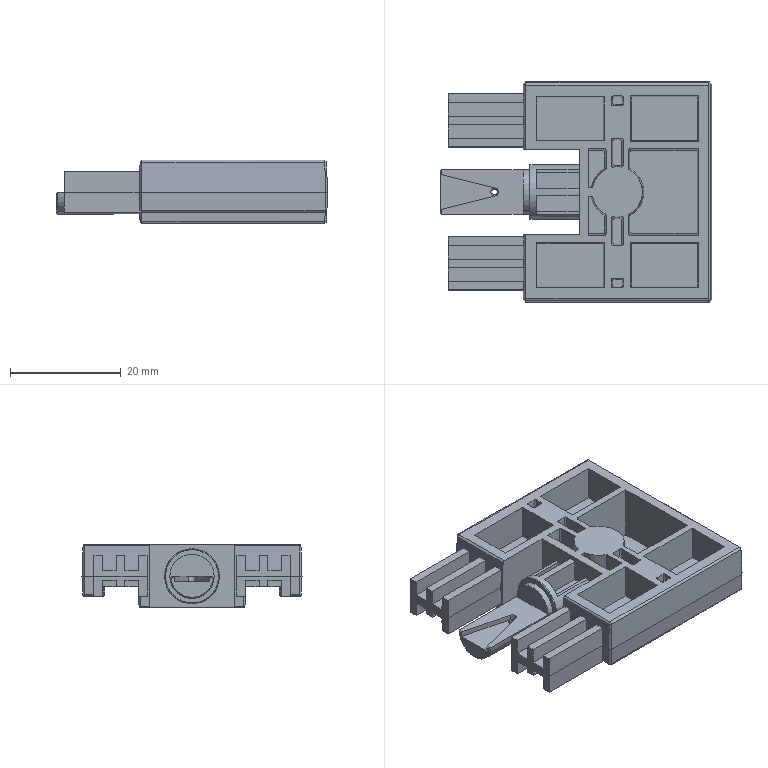Part | NX | features solid 2 | 1 solid | 278 faces | box 48.9 x 39.7 x 11.5 mm | volume 8134 mm3 | plane 199 | cylinder 45 | spline 20 | cone 12 | torus 2 | commonest cylinder face diameters 0.6 x28 0.8 x8 1.05 x2 6 x2 8 x2 9.9 x2